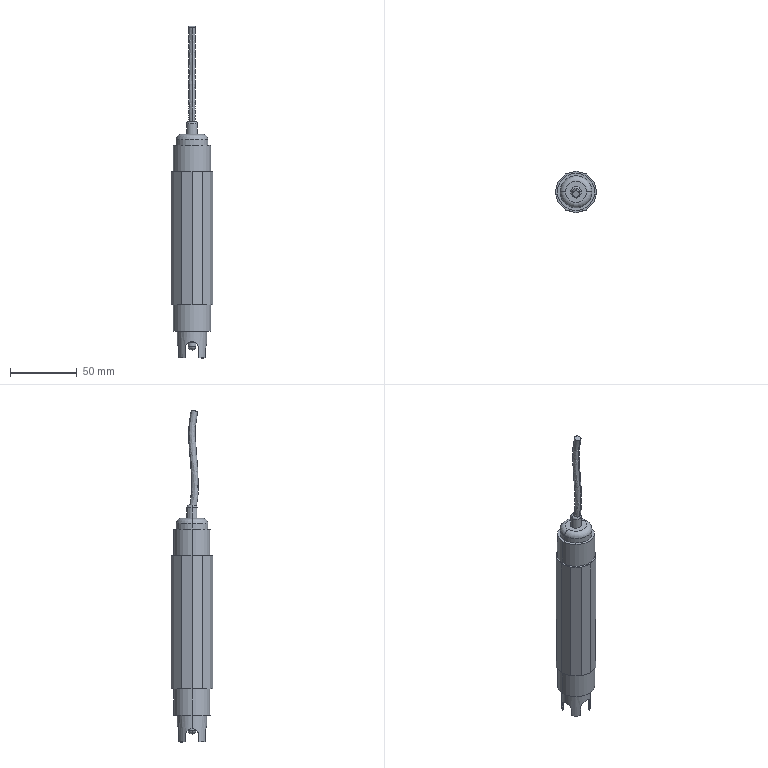Part | SolidWorks | features BaseBody 5 | 5 solids | 64 faces | box 31.058 x 31.058 x 249.412 mm | volume 105798 mm3 | plane 36 | cylinder 20 | spline 4 | torus 2 | sphere 2 | commonest cylinder face diameters 10 x4 20 x4 28 x4 6 x2 8 x2 22 x2